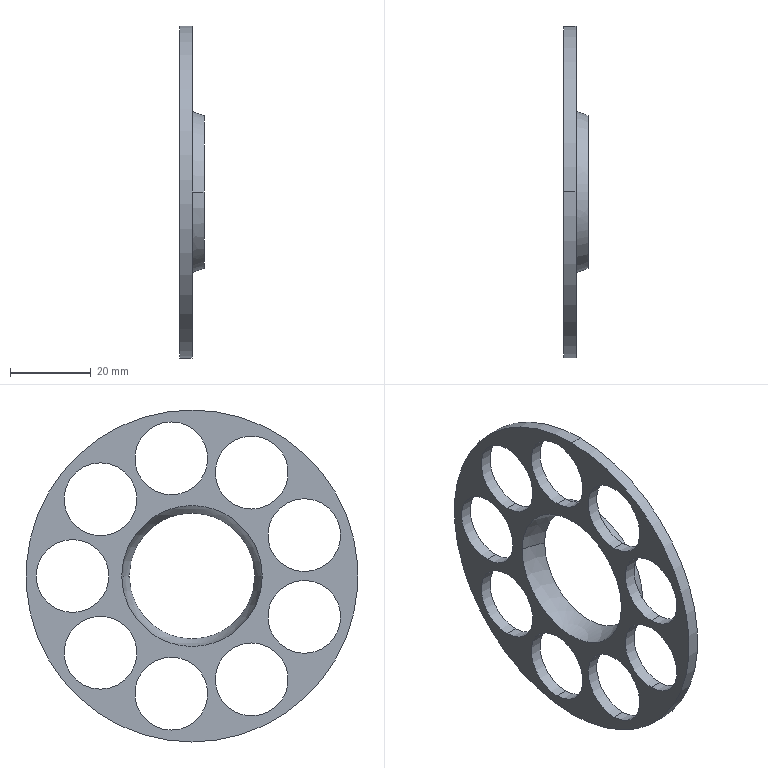Part | SolidWorks | features ICE 1, RevCut 1, Revolution 1 | 1 solid | 27 faces | box 6 x 82 x 82 mm | volume 7292 mm3 | cylinder 20 | sphere 4 | plane 3 | commonest cylinder face diameters 18 x18 82 x2
STEP:
#1=CARTESIAN_POINT('',(0.,5.123,38.052));
#2=VERTEX_POINT('',#1);
#3=CARTESIAN_POINT('',(0.,5.123,20.052));
#4=VERTEX_POINT('',#3);
#5=CARTESIAN_POINT('',(0.,5.123,29.052));
#6=DIRECTION('',(1.,0.,0.));
#7=DIRECTION('',(0.,0.,-1.));
#8=AXIS2_PLACEMENT_3D('',#5,#6,#7);
#9=CIRCLE('',#8,9.);
#10=EDGE_CURVE('',#2,#4,#9,.T.);
#11=ORIENTED_EDGE('',*,*,#10,.F.);
#12=CARTESIAN_POINT('',(3.,5.123,38.052));
#13=VERTEX_POINT('',#12);
#14=CARTESIAN_POINT('',(-7.,5.123,38.052));
#15=DIRECTION('',(1.,0.,0.));
#16=VECTOR('',#15,1000.);
#17=LINE('',#14,#16);
#18=EDGE_CURVE('',#2,#13,#17,.T.);
#19=ORIENTED_EDGE('',*,*,#18,.T.);
#20=CARTESIAN_POINT('',(3.,5.123,20.052));
#21=VERTEX_POINT('',#20);
#22=CARTESIAN_POINT('',(3.,5.123,29.052));
#23=DIRECTION('',(1.,0.,0.));
#24=DIRECTION('',(0.,0.,-1.));
#25=AXIS2_PLACEMENT_3D('',#22,#23,#24);
#26=CIRCLE('',#25,9.);
#27=EDGE_CURVE('',#13,#21,#26,.T.);
#28=ORIENTED_EDGE('',*,*,#27,.T.);
#29=CARTESIAN_POINT('',(-7.,5.123,20.052));
#30=DIRECTION('',(1.,0.,0.));
#31=VECTOR('',#30,1000.);
#32=LINE('',#29,#31);
#33=EDGE_CURVE('',#4,#21,#32,.T.);
#34=ORIENTED_EDGE('',*,*,#33,.F.);
#35=EDGE_LOOP('',(#11,#19,#28,#34));
#36=FACE_OUTER_BOUND('',#35,.T.);
#37=CARTESIAN_POINT('',(-7.,5.123,29.052));
#38=DIRECTION('',(1.,0.,0.));
#39=DIRECTION('',(0.,0.,-1.));
#40=AXIS2_PLACEMENT_3D('',#37,#38,#39);
#41=CYLINDRICAL_SURFACE('',#40,9.);
#42=ADVANCED_FACE('',(#36),#41,.F.);
#43=CARTESIAN_POINT('',(0.,22.598,27.962));
#44=VERTEX_POINT('',#43);
#45=CARTESIAN_POINT('',(0.,22.598,9.962));
#46=VERTEX_POINT('',#45);
#47=CARTESIAN_POINT('',(0.,22.598,18.962));
#48=DIRECTION('',(1.,0.,0.));
#49=DIRECTION('',(0.,0.,-1.));
#50=AXIS2_PLACEMENT_3D('',#47,#48,#49);
#51=CIRCLE('',#50,9.);
#52=EDGE_CURVE('',#44,#46,#51,.T.);
#53=ORIENTED_EDGE('',*,*,#52,.F.);
#54=CARTESIAN_POINT('',(3.,22.598,27.962));
#55=VERTEX_POINT('',#54);
#56=CARTESIAN_POINT('',(-7.,22.598,27.962));
#57=DIRECTION('',(1.,0.,0.));
#58=VECTOR('',#57,1000.);
#59=LINE('',#56,#58);
#60=EDGE_CURVE('',#44,#55,#59,.T.);
#61=ORIENTED_EDGE('',*,*,#60,.T.);
#62=CARTESIAN_POINT('',(3.,22.598,9.962));
#63=VERTEX_POINT('',#62);
#64=CARTESIAN_POINT('',(3.,22.598,18.962));
#65=DIRECTION('',(1.,0.,0.));
#66=DIRECTION('',(0.,0.,-1.));
#67=AXIS2_PLACEMENT_3D('',#64,#65,#66);
#68=CIRCLE('',#67,9.);
#69=EDGE_CURVE('',#55,#63,#68,.T.);
#70=ORIENTED_EDGE('',*,*,#69,.T.);
#71=CARTESIAN_POINT('',(-7.,22.598,9.962));
#72=DIRECTION('',(1.,0.,0.));
#73=VECTOR('',#72,1000.);
#74=LINE('',#71,#73);
#75=EDGE_CURVE('',#46,#63,#74,.T.);
#76=ORIENTED_EDGE('',*,*,#75,.F.);
#77=EDGE_LOOP('',(#53,#61,#70,#76));
#78=FACE_OUTER_BOUND('',#77,.T.);
#79=CARTESIAN_POINT('',(-7.,22.598,18.962));
#80=DIRECTION('',(1.,0.,0.));
#81=DIRECTION('',(0.,0.,-1.));
#82=AXIS2_PLACEMENT_3D('',#79,#80,#81);
#83=CYLINDRICAL_SURFACE('',#82,9.);
#84=ADVANCED_FACE('',(#78),#83,.F.);
#85=CARTESIAN_POINT('',(0.,-27.721,19.09));
#86=VERTEX_POINT('',#85);
#87=CARTESIAN_POINT('',(0.,-27.721,1.09));
#88=VERTEX_POINT('',#87);
#89=CARTESIAN_POINT('',(0.,-27.721,10.09));
#90=DIRECTION('',(1.,0.,0.));
#91=DIRECTION('',(0.,0.,-1.));
#92=AXIS2_PLACEMENT_3D('',#89,#90,#91);
#93=CIRCLE('',#92,9.);
#94=EDGE_CURVE('',#86,#88,#93,.T.);
#95=ORIENTED_EDGE('',*,*,#94,.F.);
#96=CARTESIAN_POINT('',(3.,-27.721,19.09));
#97=VERTEX_POINT('',#96);
#98=CARTESIAN_POINT('',(-7.,-27.721,19.09));
#99=DIRECTION('',(1.,0.,0.));
#100=VECTOR('',#99,1000.);
#101=LINE('',#98,#100);
#102=EDGE_CURVE('',#86,#97,#101,.T.);
#103=ORIENTED_EDGE('',*,*,#102,.T.);
#104=CARTESIAN_POINT('',(3.,-27.721,1.09));
#105=VERTEX_POINT('',#104);
#106=CARTESIAN_POINT('',(3.,-27.721,10.09));
#107=DIRECTION('',(1.,0.,0.));
#108=DIRECTION('',(0.,0.,-1.));
#109=AXIS2_PLACEMENT_3D('',#106,#107,#108);
#110=CIRCLE('',#109,9.);
#111=EDGE_CURVE('',#97,#105,#110,.T.);
#112=ORIENTED_EDGE('',*,*,#111,.T.);
#113=CARTESIAN_POINT('',(-7.,-27.721,1.09));
#114=DIRECTION('',(1.,0.,0.));
#115=VECTOR('',#114,1000.);
#116=LINE('',#113,#115);
#117=EDGE_CURVE('',#88,#105,#116,.T.);
#118=ORIENTED_EDGE('',*,*,#117,.F.);
#119=EDGE_LOOP('',(#95,#103,#112,#118));
#120=FACE_OUTER_BOUND('',#119,.T.);
#121=CARTESIAN_POINT('',(-7.,-27.721,10.09));
#122=DIRECTION('',(1.,0.,0.));
#123=DIRECTION('',(0.,0.,-1.));
#124=AXIS2_PLACEMENT_3D('',#121,#122,#123);
#125=CYLINDRICAL_SURFACE('',#124,9.);
#126=ADVANCED_FACE('',(#120),#125,.F.);
#127=CARTESIAN_POINT('',(0.,-14.75,34.548));
#128=VERTEX_POINT('',#127);
#129=CARTESIAN_POINT('',(0.,-14.75,16.548));
#130=VERTEX_POINT('',#129);
#131=CARTESIAN_POINT('',(0.,-14.75,25.548));
#132=DIRECTION('',(1.,0.,0.));
#133=DIRECTION('',(0.,0.,-1.));
#134=AXIS2_PLACEMENT_3D('',#131,#132,#133);
#135=CIRCLE('',#134,9.);
#136=EDGE_CURVE('',#128,#130,#135,.T.);
#137=ORIENTED_EDGE('',*,*,#136,.F.);
#138=CARTESIAN_POINT('',(3.,-14.75,34.548));
#139=VERTEX_POINT('',#138);
#140=CARTESIAN_POINT('',(-7.,-14.75,34.548));
#141=DIRECTION('',(1.,0.,0.));
#142=VECTOR('',#141,1000.);
#143=LINE('',#140,#142);
#144=EDGE_CURVE('',#128,#139,#143,.T.);
#145=ORIENTED_EDGE('',*,*,#144,.T.);
#146=CARTESIAN_POINT('',(3.,-14.75,16.548));
#147=VERTEX_POINT('',#146);
#148=CARTESIAN_POINT('',(3.,-14.75,25.548));
#149=DIRECTION('',(1.,0.,0.));
#150=DIRECTION('',(0.,0.,-1.));
#151=AXIS2_PLACEMENT_3D('',#148,#149,#150);
#152=CIRCLE('',#151,9.);
#153=EDGE_CURVE('',#139,#147,#152,.T.);
#154=ORIENTED_EDGE('',*,*,#153,.T.);
#155=CARTESIAN_POINT('',(-7.,-14.75,16.548));
#156=DIRECTION('',(1.,0.,0.));
#157=VECTOR('',#156,1000.);
#158=LINE('',#155,#157);
#159=EDGE_CURVE('',#130,#147,#158,.T.);
#160=ORIENTED_EDGE('',*,*,#159,.F.);
#161=EDGE_LOOP('',(#137,#145,#154,#160));
#162=FACE_OUTER_BOUND('',#161,.T.);
#163=CARTESIAN_POINT('',(-7.,-14.75,25.548));
#164=DIRECTION('',(1.,0.,0.));
#165=DIRECTION('',(0.,0.,-1.));
#166=AXIS2_PLACEMENT_3D('',#163,#164,#165);
#167=CYLINDRICAL_SURFACE('',#166,9.);
#168=ADVANCED_FACE('',(#162),#167,.F.);
#169=CARTESIAN_POINT('',(0.,-14.75,-16.548));
#170=VERTEX_POINT('',#169);
#171=CARTESIAN_POINT('',(0.,-14.75,-34.548));
#172=VERTEX_POINT('',#171);
#173=CARTESIAN_POINT('',(0.,-14.75,-25.548));
#174=DIRECTION('',(1.,0.,0.));
#175=DIRECTION('',(0.,0.,-1.));
#176=AXIS2_PLACEMENT_3D('',#173,#174,#175);
#177=CIRCLE('',#176,9.);
#178=EDGE_CURVE('',#170,#172,#177,.T.);
#179=ORIENTED_EDGE('',*,*,#178,.F.);
#180=CARTESIAN_POINT('',(3.,-14.75,-16.548));
#181=VERTEX_POINT('',#180);
#182=CARTESIAN_POINT('',(-7.,-14.75,-16.548));
#183=DIRECTION('',(1.,0.,0.));
#184=VECTOR('',#183,1000.);
#185=LINE('',#182,#184);
#186=EDGE_CURVE('',#170,#181,#185,.T.);
#187=ORIENTED_EDGE('',*,*,#186,.T.);
#188=CARTESIAN_POINT('',(3.,-14.75,-34.548));
#189=VERTEX_POINT('',#188);
#190=CARTESIAN_POINT('',(3.,-14.75,-25.548));
#191=DIRECTION('',(1.,0.,0.));
#192=DIRECTION('',(0.,0.,-1.));
#193=AXIS2_PLACEMENT_3D('',#190,#191,#192);
#194=CIRCLE('',#193,9.);
#195=EDGE_CURVE('',#181,#189,#194,.T.);
#196=ORIENTED_EDGE('',*,*,#195,.T.);
#197=CARTESIAN_POINT('',(-7.,-14.75,-34.548));
#198=DIRECTION('',(1.,0.,0.));
#199=VECTOR('',#198,1000.);
#200=LINE('',#197,#199);
#201=EDGE_CURVE('',#172,#189,#200,.T.);
#202=ORIENTED_EDGE('',*,*,#201,.F.);
#203=EDGE_LOOP('',(#179,#187,#196,#202));
#204=FACE_OUTER_BOUND('',#203,.T.);
#205=CARTESIAN_POINT('',(-7.,-14.75,-25.548));
#206=DIRECTION('',(1.,0.,0.));
#207=DIRECTION('',(0.,0.,-1.));
#208=AXIS2_PLACEMENT_3D('',#205,#206,#207);
#209=CYLINDRICAL_SURFACE('',#208,9.);
#210=ADVANCED_FACE('',(#204),#209,.F.);
#211=CARTESIAN_POINT('',(0.,-27.721,-1.09));
#212=VERTEX_POINT('',#211);
#213=CARTESIAN_POINT('',(0.,-27.721,-19.09));
#214=VERTEX_POINT('',#213);
#215=CARTESIAN_POINT('',(0.,-27.721,-10.09));
#216=DIRECTION('',(1.,0.,0.));
#217=DIRECTION('',(0.,0.,-1.));
#218=AXIS2_PLACEMENT_3D('',#215,#216,#217);
#219=CIRCLE('',#218,9.);
#220=EDGE_CURVE('',#212,#214,#219,.T.);
#221=ORIENTED_EDGE('',*,*,#220,.F.);
#222=CARTESIAN_POINT('',(3.,-27.721,-1.09));
#223=VERTEX_POINT('',#222);
#224=CARTESIAN_POINT('',(-7.,-27.721,-1.09));
#225=DIRECTION('',(1.,0.,0.));
#226=VECTOR('',#225,1000.);
#227=LINE('',#224,#226);
#228=EDGE_CURVE('',#212,#223,#227,.T.);
#229=ORIENTED_EDGE('',*,*,#228,.T.);
#230=CARTESIAN_POINT('',(3.,-27.721,-19.09));
#231=VERTEX_POINT('',#230);
#232=CARTESIAN_POINT('',(3.,-27.721,-10.09));
#233=DIRECTION('',(1.,0.,0.));
#234=DIRECTION('',(0.,0.,-1.));
#235=AXIS2_PLACEMENT_3D('',#232,#233,#234);
#236=CIRCLE('',#235,9.);
#237=EDGE_CURVE('',#223,#231,#236,.T.);
#238=ORIENTED_EDGE('',*,*,#237,.T.);
#239=CARTESIAN_POINT('',(-7.,-27.721,-19.09));
#240=DIRECTION('',(1.,0.,0.));
#241=VECTOR('',#240,1000.);
#242=LINE('',#239,#241);
#243=EDGE_CURVE('',#214,#231,#242,.T.);
#244=ORIENTED_EDGE('',*,*,#243,.F.);
#245=EDGE_LOOP('',(#221,#229,#238,#244));
#246=FACE_OUTER_BOUND('',#245,.T.);
#247=CARTESIAN_POINT('',(-7.,-27.721,-10.09));
#248=DIRECTION('',(1.,0.,0.));
#249=DIRECTION('',(0.,0.,-1.));
#250=AXIS2_PLACEMENT_3D('',#247,#248,#249);
#251=CYLINDRICAL_SURFACE('',#250,9.);
#252=ADVANCED_FACE('',(#246),#251,.F.);
#253=CARTESIAN_POINT('',(0.,22.598,-9.962));
#254=VERTEX_POINT('',#253);
#255=CARTESIAN_POINT('',(0.,22.598,-27.962));
#256=VERTEX_POINT('',#255);
#257=CARTESIAN_POINT('',(0.,22.598,-18.962));
#258=DIRECTION('',(1.,0.,0.));
#259=DIRECTION('',(0.,0.,-1.));
#260=AXIS2_PLACEMENT_3D('',#257,#258,#259);
#261=CIRCLE('',#260,9.);
#262=EDGE_CURVE('',#254,#256,#261,.T.);
#263=ORIENTED_EDGE('',*,*,#262,.F.);
#264=CARTESIAN_POINT('',(3.,22.598,-9.962));
#265=VERTEX_POINT('',#264);
#266=CARTESIAN_POINT('',(-7.,22.598,-9.962));
#267=DIRECTION('',(1.,0.,0.));
#268=VECTOR('',#267,1000.);
#269=LINE('',#266,#268);
#270=EDGE_CURVE('',#254,#265,#269,.T.);
#271=ORIENTED_EDGE('',*,*,#270,.T.);
#272=CARTESIAN_POINT('',(3.,22.598,-27.962));
#273=VERTEX_POINT('',#272);
#274=CARTESIAN_POINT('',(3.,22.598,-18.962));
#275=DIRECTION('',(1.,0.,0.));
#276=DIRECTION('',(0.,0.,-1.));
#277=AXIS2_PLACEMENT_3D('',#274,#275,#276);
#278=CIRCLE('',#277,9.);
#279=EDGE_CURVE('',#265,#273,#278,.T.);
#280=ORIENTED_EDGE('',*,*,#279,.T.);
#281=CARTESIAN_POINT('',(-7.,22.598,-27.962));
#282=DIRECTION('',(1.,0.,0.));
#283=VECTOR('',#282,1000.);
#284=LINE('',#281,#283);
#285=EDGE_CURVE('',#256,#273,#284,.T.);
#286=ORIENTED_EDGE('',*,*,#285,.F.);
#287=EDGE_LOOP('',(#263,#271,#280,#286));
#288=FACE_OUTER_BOUND('',#287,.T.);
#289=CARTESIAN_POINT('',(-7.,22.598,-18.962));
#290=DIRECTION('',(1.,0.,0.));
#291=DIRECTION('',(0.,0.,-1.));
#292=AXIS2_PLACEMENT_3D('',#289,#290,#291);
#293=CYLINDRICAL_SURFACE('',#292,9.);
#294=ADVANCED_FACE('',(#288),#293,.F.);
#295=CARTESIAN_POINT('',(0.,5.123,-20.052));
#296=VERTEX_POINT('',#295);
#297=CARTESIAN_POINT('',(0.,5.123,-38.052));
#298=VERTEX_POINT('',#297);
#299=CARTESIAN_POINT('',(0.,5.123,-29.052));
#300=DIRECTION('',(1.,0.,0.));
#301=DIRECTION('',(0.,0.,-1.));
#302=AXIS2_PLACEMENT_3D('',#299,#300,#301);
#303=CIRCLE('',#302,9.);
#304=EDGE_CURVE('',#296,#298,#303,.T.);
#305=ORIENTED_EDGE('',*,*,#304,.F.);
#306=CARTESIAN_POINT('',(3.,5.123,-20.052));
#307=VERTEX_POINT('',#306);
#308=CARTESIAN_POINT('',(-7.,5.123,-20.052));
#309=DIRECTION('',(1.,0.,0.));
#310=VECTOR('',#309,1000.);
#311=LINE('',#308,#310);
#312=EDGE_CURVE('',#296,#307,#311,.T.);
#313=ORIENTED_EDGE('',*,*,#312,.T.);
#314=CARTESIAN_POINT('',(3.,5.123,-38.052));
#315=VERTEX_POINT('',#314);
#316=CARTESIAN_POINT('',(3.,5.123,-29.052));
#317=DIRECTION('',(1.,0.,0.));
#318=DIRECTION('',(0.,0.,-1.));
#319=AXIS2_PLACEMENT_3D('',#316,#317,#318);
#320=CIRCLE('',#319,9.);
#321=EDGE_CURVE('',#307,#315,#320,.T.);
#322=ORIENTED_EDGE('',*,*,#321,.T.);
#323=CARTESIAN_POINT('',(-7.,5.123,-38.052));
#324=DIRECTION('',(1.,0.,0.));
#325=VECTOR('',#324,1000.);
#326=LINE('',#323,#325);
#327=EDGE_CURVE('',#298,#315,#326,.T.);
#328=ORIENTED_EDGE('',*,*,#327,.F.);
#329=EDGE_LOOP('',(#305,#313,#322,#328));
#330=FACE_OUTER_BOUND('',#329,.T.);
#331=CARTESIAN_POINT('',(-7.,5.123,-29.052));
#332=DIRECTION('',(1.,0.,0.));
#333=DIRECTION('',(0.,0.,-1.));
#334=AXIS2_PLACEMENT_3D('',#331,#332,#333);
#335=CYLINDRICAL_SURFACE('',#334,9.);
#336=ADVANCED_FACE('',(#330),#335,.F.);
#337=CARTESIAN_POINT('',(0.,29.5,9.));
#338=VERTEX_POINT('',#337);
#339=CARTESIAN_POINT('',(0.,29.5,-9.));
#340=VERTEX_POINT('',#339);
#341=CARTESIAN_POINT('',(0.,29.5,0.));
#342=DIRECTION('',(1.,0.,0.));
#343=DIRECTION('',(0.,0.,-1.));
#344=AXIS2_PLACEMENT_3D('',#341,#342,#343);
#345=CIRCLE('',#344,9.);
#346=EDGE_CURVE('',#338,#340,#345,.T.);
#347=ORIENTED_EDGE('',*,*,#346,.F.);
#348=CARTESIAN_POINT('',(3.,29.5,9.));
#349=VERTEX_POINT('',#348);
#350=CARTESIAN_POINT('',(-7.,29.5,9.));
#351=DIRECTION('',(1.,0.,0.));
#352=VECTOR('',#351,1000.);
#353=LINE('',#350,#352);
#354=EDGE_CURVE('',#338,#349,#353,.T.);
#355=ORIENTED_EDGE('',*,*,#354,.T.);
#356=CARTESIAN_POINT('',(3.,29.5,-9.));
#357=VERTEX_POINT('',#356);
#358=CARTESIAN_POINT('',(3.,29.5,0.));
#359=DIRECTION('',(1.,0.,0.));
#360=DIRECTION('',(0.,0.,-1.));
#361=AXIS2_PLACEMENT_3D('',#358,#359,#360);
#362=CIRCLE('',#361,9.);
#363=EDGE_CURVE('',#349,#357,#362,.T.);
#364=ORIENTED_EDGE('',*,*,#363,.T.);
#365=CARTESIAN_POINT('',(-7.,29.5,-9.));
#366=DIRECTION('',(1.,0.,0.));
#367=VECTOR('',#366,1000.);
#368=LINE('',#365,#367);
#369=EDGE_CURVE('',#340,#357,#368,.T.);
#370=ORIENTED_EDGE('',*,*,#369,.F.);
#371=EDGE_LOOP('',(#347,#355,#364,#370));
#372=FACE_OUTER_BOUND('',#371,.T.);
#373=CARTESIAN_POINT('',(-7.,29.5,0.));
#374=DIRECTION('',(1.,0.,0.));
#375=DIRECTION('',(0.,0.,-1.));
#376=AXIS2_PLACEMENT_3D('',#373,#374,#375);
#377=CYLINDRICAL_SURFACE('',#376,9.);
#378=ADVANCED_FACE('',(#372),#377,.F.);
#379=CARTESIAN_POINT('',(0.,-17.371,0.));
#380=VERTEX_POINT('',#379);
#381=CARTESIAN_POINT('',(0.,17.371,0.));
#382=VERTEX_POINT('',#381);
#383=CARTESIAN_POINT('',(0.,0.,0.));
#384=DIRECTION('',(1.,0.,0.));
#385=DIRECTION('',(0.,0.,-1.));
#386=AXIS2_PLACEMENT_3D('',#383,#384,#385);
#387=CIRCLE('',#386,17.371);
#388=EDGE_CURVE('',#380,#382,#387,.T.);
#389=ORIENTED_EDGE('',*,*,#388,.F.);
#390=CARTESIAN_POINT('',(6.,-15.5,0.));
#391=VERTEX_POINT('',#390);
#392=CARTESIAN_POINT('',(-2.124,0.,0.));
#393=DIRECTION('',(0.,0.,1.));
#394=DIRECTION('',(0.,-1.,0.));
#395=AXIS2_PLACEMENT_3D('',#392,#393,#394);
#396=CIRCLE('',#395,17.5);
#397=EDGE_CURVE('',#380,#391,#396,.T.);
#398=ORIENTED_EDGE('',*,*,#397,.T.);
#399=CARTESIAN_POINT('',(6.,15.5,0.));
#400=VERTEX_POINT('',#399);
#401=CARTESIAN_POINT('',(6.,0.,0.));
#402=DIRECTION('',(1.,0.,0.));
#403=DIRECTION('',(0.,0.,-1.));
#404=AXIS2_PLACEMENT_3D('',#401,#402,#403);
#405=CIRCLE('',#404,15.5);
#406=EDGE_CURVE('',#391,#400,#405,.T.);
#407=ORIENTED_EDGE('',*,*,#406,.T.);
#408=CARTESIAN_POINT('',(-2.124,0.,0.));
#409=DIRECTION('',(0.,0.,-1.));
#410=DIRECTION('',(-1.,0.,0.));
#411=AXIS2_PLACEMENT_3D('',#408,#409,#410);
#412=CIRCLE('',#411,17.5);
#413=EDGE_CURVE('',#382,#400,#412,.T.);
#414=ORIENTED_EDGE('',*,*,#413,.F.);
#415=EDGE_LOOP('',(#389,#398,#407,#414));
#416=FACE_OUTER_BOUND('',#415,.T.);
#417=CARTESIAN_POINT('',(-2.124,0.,0.));
#418=DIRECTION('',(0.,0.,1.));
#419=DIRECTION('',(0.,1.,0.));
#420=AXIS2_PLACEMENT_3D('',#417,#418,#419);
#421=SPHERICAL_SURFACE('',#420,17.5);
#422=ADVANCED_FACE('',(#416),#421,.F.);
#423=CARTESIAN_POINT('',(3.,0.,41.));
#424=VERTEX_POINT('',#423);
#425=CARTESIAN_POINT('',(3.,0.,-41.));
#426=VERTEX_POINT('',#425);
#427=CARTESIAN_POINT('',(3.,0.,0.));
#428=DIRECTION('',(-1.,0.,0.));
#429=DIRECTION('',(0.,0.,1.));
#430=AXIS2_PLACEMENT_3D('',#427,#428,#429);
#431=CIRCLE('',#430,41.);
#432=EDGE_CURVE('',#424,#426,#431,.T.);
#433=ORIENTED_EDGE('',*,*,#432,.T.);
#434=CARTESIAN_POINT('',(0.,0.,-41.));
#435=VERTEX_POINT('',#434);
#436=CARTESIAN_POINT('',(0.,0.,-41.));
#437=DIRECTION('',(-1.,0.,0.));
#438=VECTOR('',#437,1000.);
#439=LINE('',#436,#438);
#440=EDGE_CURVE('',#426,#435,#439,.T.);
#441=ORIENTED_EDGE('',*,*,#440,.T.);
#442=CARTESIAN_POINT('',(0.,0.,41.));
#443=VERTEX_POINT('',#442);
#444=CARTESIAN_POINT('',(0.,0.,0.));
#445=DIRECTION('',(-1.,0.,0.));
#446=DIRECTION('',(0.,0.,1.));
#447=AXIS2_PLACEMENT_3D('',#444,#445,#446);
#448=CIRCLE('',#447,41.);
#449=EDGE_CURVE('',#443,#435,#448,.T.);
#450=ORIENTED_EDGE('',*,*,#449,.F.);
#451=CARTESIAN_POINT('',(0.,0.,41.));
#452=DIRECTION('',(-1.,0.,0.));
#453=VECTOR('',#452,1000.);
#454=LINE('',#451,#453);
#455=EDGE_CURVE('',#424,#443,#454,.T.);
#456=ORIENTED_EDGE('',*,*,#455,.F.);
#457=EDGE_LOOP('',(#433,#441,#450,#456));
#458=FACE_OUTER_BOUND('',#457,.T.);
#459=CARTESIAN_POINT('',(0.,0.,0.));
#460=DIRECTION('',(-1.,0.,0.));
#461=DIRECTION('',(0.,0.,1.));
#462=AXIS2_PLACEMENT_3D('',#459,#460,#461);
#463=CYLINDRICAL_SURFACE('',#462,41.);
#464=ADVANCED_FACE('',(#458),#463,.T.);
#465=CARTESIAN_POINT('',(6.,18.822,0.));
#466=VERTEX_POINT('',#465);
#467=CARTESIAN_POINT('',(6.,-18.822,0.));
#468=VERTEX_POINT('',#467);
#469=CARTESIAN_POINT('',(6.,0.,0.));
#470=DIRECTION('',(-1.,0.,0.));
#471=DIRECTION('',(0.,0.,1.));
#472=AXIS2_PLACEMENT_3D('',#469,#470,#471);
#473=CIRCLE('',#472,18.822);
#474=EDGE_CURVE('',#466,#468,#473,.T.);
#475=ORIENTED_EDGE('',*,*,#474,.T.);
#476=CARTESIAN_POINT('',(3.,-19.849,0.));
#477=VERTEX_POINT('',#476);
#478=CARTESIAN_POINT('',(-2.124,0.,0.));
#479=DIRECTION('',(0.,0.,-1.));
#480=DIRECTION('',(0.,1.,0.));
#481=AXIS2_PLACEMENT_3D('',#478,#479,#480);
#482=CIRCLE('',#481,20.5);
#483=EDGE_CURVE('',#468,#477,#482,.T.);
#484=ORIENTED_EDGE('',*,*,#483,.T.);
#485=CARTESIAN_POINT('',(3.,19.849,0.));
#486=VERTEX_POINT('',#485);
#487=CARTESIAN_POINT('',(3.,0.,0.));
#488=DIRECTION('',(-1.,0.,0.));
#489=DIRECTION('',(0.,0.,1.));
#490=AXIS2_PLACEMENT_3D('',#487,#488,#489);
#491=CIRCLE('',#490,19.849);
#492=EDGE_CURVE('',#486,#477,#491,.T.);
#493=ORIENTED_EDGE('',*,*,#492,.F.);
#494=CARTESIAN_POINT('',(-2.124,0.,0.));
#495=DIRECTION('',(0.,0.,1.));
#496=DIRECTION('',(1.,0.,0.));
#497=AXIS2_PLACEMENT_3D('',#494,#495,#496);
#498=CIRCLE('',#497,20.5);
#499=EDGE_CURVE('',#466,#486,#498,.T.);
#500=ORIENTED_EDGE('',*,*,#499,.F.);
#501=EDGE_LOOP('',(#475,#484,#493,#500));
#502=FACE_OUTER_BOUND('',#501,.T.);
#503=CARTESIAN_POINT('',(-2.124,0.,0.));
#504=DIRECTION('',(0.,0.,-1.));
#505=DIRECTION('',(0.,1.,0.));
#506=AXIS2_PLACEMENT_3D('',#503,#504,#505);
#507=SPHERICAL_SURFACE('',#506,20.5);
#508=ADVANCED_FACE('',(#502),#507,.T.);
#509=CARTESIAN_POINT('',(6.,0.,0.));
#510=DIRECTION('',(1.,0.,0.));
#511=DIRECTION('',(0.,0.,-1.));
#512=AXIS2_PLACEMENT_3D('',#509,#510,#511);
#513=CIRCLE('',#512,15.5);
#514=EDGE_CURVE('',#400,#391,#513,.T.);
#515=ORIENTED_EDGE('',*,*,#514,.F.);
#516=ORIENTED_EDGE('',*,*,#406,.F.);
#517=EDGE_LOOP('',(#515,#516));
#518=FACE_BOUND('',#517,.T.);
#519=ORIENTED_EDGE('',*,*,#474,.F.);
#520=CARTESIAN_POINT('',(6.,0.,0.));
#521=DIRECTION('',(-1.,0.,0.));
#522=DIRECTION('',(0.,0.,1.));
#523=AXIS2_PLACEMENT_3D('',#520,#521,#522);
#524=CIRCLE('',#523,18.822);
#525=EDGE_CURVE('',#468,#466,#524,.T.);
#526=ORIENTED_EDGE('',*,*,#525,.F.);
#527=EDGE_LOOP('',(#519,#526));
#528=FACE_OUTER_BOUND('',#527,.T.);
#529=CARTESIAN_POINT('',(6.,0.,0.));
#530=DIRECTION('',(-1.,0.,0.));
#531=DIRECTION('',(0.,0.,1.));
#532=AXIS2_PLACEMENT_3D('',#529,#530,#531);
#533=PLANE('',#532);
#534=ADVANCED_FACE('',(#518,#528),#533,.F.);
#535=ORIENTED_EDGE('',*,*,#483,.F.);
#536=ORIENTED_EDGE('',*,*,#525,.T.);
#537=ORIENTED_EDGE('',*,*,#499,.T.);
#538=CARTESIAN_POINT('',(3.,0.,0.));
#539=DIRECTION('',(-1.,0.,0.));
#540=DIRECTION('',(0.,0.,1.));
#541=AXIS2_PLACEMENT_3D('',#538,#539,#540);
#542=CIRCLE('',#541,19.849);
#543=EDGE_CURVE('',#477,#486,#542,.T.);
#544=ORIENTED_EDGE('',*,*,#543,.F.);
#545=EDGE_LOOP('',(#535,#536,#537,#544));
#546=FACE_OUTER_BOUND('',#545,.T.);
#547=CARTESIAN_POINT('',(-2.124,0.,0.));
#548=DIRECTION('',(0.,0.,-1.));
#549=DIRECTION('',(0.,1.,0.));
#550=AXIS2_PLACEMENT_3D('',#547,#548,#549);
#551=SPHERICAL_SURFACE('',#550,20.5);
#552=ADVANCED_FACE('',(#546),#551,.T.);
#553=CARTESIAN_POINT('',(3.,5.123,29.052));
#554=DIRECTION('',(1.,0.,0.));
#555=DIRECTION('',(0.,0.,-1.));
#556=AXIS2_PLACEMENT_3D('',#553,#554,#555);
#557=CIRCLE('',#556,9.);
#558=EDGE_CURVE('',#21,#13,#557,.T.);
#559=ORIENTED_EDGE('',*,*,#558,.F.);
#560=ORIENTED_EDGE('',*,*,#27,.F.);
#561=EDGE_LOOP('',(#559,#560));
#562=FACE_BOUND('',#561,.T.);
#563=CARTESIAN_POINT('',(3.,22.598,18.962));
#564=DIRECTION('',(1.,0.,0.));
#565=DIRECTION('',(0.,0.,-1.));
#566=AXIS2_PLACEMENT_3D('',#563,#564,#565);
#567=CIRCLE('',#566,9.);
#568=EDGE_CURVE('',#63,#55,#567,.T.);
#569=ORIENTED_EDGE('',*,*,#568,.F.);
#570=ORIENTED_EDGE('',*,*,#69,.F.);
#571=EDGE_LOOP('',(#569,#570));
#572=FACE_BOUND('',#571,.T.);
#573=CARTESIAN_POINT('',(3.,-27.721,10.09));
#574=DIRECTION('',(1.,0.,0.));
#575=DIRECTION('',(0.,0.,-1.));
#576=AXIS2_PLACEMENT_3D('',#573,#574,#575);
#577=CIRCLE('',#576,9.);
#578=EDGE_CURVE('',#105,#97,#577,.T.);
#579=ORIENTED_EDGE('',*,*,#578,.F.);
#580=ORIENTED_EDGE('',*,*,#111,.F.);
#581=EDGE_LOOP('',(#579,#580));
#582=FACE_BOUND('',#581,.T.);
#583=CARTESIAN_POINT('',(3.,-14.75,25.548));
#584=DIRECTION('',(1.,0.,0.));
#585=DIRECTION('',(0.,0.,-1.));
#586=AXIS2_PLACEMENT_3D('',#583,#584,#585);
#587=CIRCLE('',#586,9.);
#588=EDGE_CURVE('',#147,#139,#587,.T.);
#589=ORIENTED_EDGE('',*,*,#588,.F.);
#590=ORIENTED_EDGE('',*,*,#153,.F.);
#591=EDGE_LOOP('',(#589,#590));
#592=FACE_BOUND('',#591,.T.);
#593=CARTESIAN_POINT('',(3.,-14.75,-25.548));
#594=DIRECTION('',(1.,0.,0.));
#595=DIRECTION('',(0.,0.,-1.));
#596=AXIS2_PLACEMENT_3D('',#593,#594,#595);
#597=CIRCLE('',#596,9.);
#598=EDGE_CURVE('',#189,#181,#597,.T.);
#599=ORIENTED_EDGE('',*,*,#598,.F.);
#600=ORIENTED_EDGE('',*,*,#195,.F.);
#601=EDGE_LOOP('',(#599,#600));
#602=FACE_BOUND('',#601,.T.);
#603=CARTESIAN_POINT('',(3.,-27.721,-10.09));
#604=DIRECTION('',(1.,0.,0.));
#605=DIRECTION('',(0.,0.,-1.));
#606=AXIS2_PLACEMENT_3D('',#603,#604,#605);
#607=CIRCLE('',#606,9.);
#608=EDGE_CURVE('',#231,#223,#607,.T.);
#609=ORIENTED_EDGE('',*,*,#608,.F.);
#610=ORIENTED_EDGE('',*,*,#237,.F.);
#611=EDGE_LOOP('',(#609,#610));
#612=FACE_BOUND('',#611,.T.);
#613=CARTESIAN_POINT('',(3.,22.598,-18.962));
#614=DIRECTION('',(1.,0.,0.));
#615=DIRECTION('',(0.,0.,-1.));
#616=AXIS2_PLACEMENT_3D('',#613,#614,#615);
#617=CIRCLE('',#616,9.);
#618=EDGE_CURVE('',#273,#265,#617,.T.);
#619=ORIENTED_EDGE('',*,*,#618,.F.);
#620=ORIENTED_EDGE('',*,*,#279,.F.);
#621=EDGE_LOOP('',(#619,#620));
#622=FACE_BOUND('',#621,.T.);
#623=CARTESIAN_POINT('',(3.,5.123,-29.052));
#624=DIRECTION('',(1.,0.,0.));
#625=DIRECTION('',(0.,0.,-1.));
#626=AXIS2_PLACEMENT_3D('',#623,#624,#625);
#627=CIRCLE('',#626,9.);
#628=EDGE_CURVE('',#315,#307,#627,.T.);
#629=ORIENTED_EDGE('',*,*,#628,.F.);
#630=ORIENTED_EDGE('',*,*,#321,.F.);
#631=EDGE_LOOP('',(#629,#630));
#632=FACE_BOUND('',#631,.T.);
#633=CARTESIAN_POINT('',(3.,29.5,0.));
#634=DIRECTION('',(1.,0.,0.));
#635=DIRECTION('',(0.,0.,-1.));
#636=AXIS2_PLACEMENT_3D('',#633,#634,#635);
#637=CIRCLE('',#636,9.);
#638=EDGE_CURVE('',#357,#349,#637,.T.);
#639=ORIENTED_EDGE('',*,*,#638,.F.);
#640=ORIENTED_EDGE('',*,*,#363,.F.);
#641=EDGE_LOOP('',(#639,#640));
#642=FACE_BOUND('',#641,.T.);
#643=ORIENTED_EDGE('',*,*,#432,.F.);
#644=CARTESIAN_POINT('',(3.,0.,0.));
#645=DIRECTION('',(-1.,0.,0.));
#646=DIRECTION('',(0.,0.,1.));
#647=AXIS2_PLACEMENT_3D('',#644,#645,#646);
#648=CIRCLE('',#647,41.);
#649=EDGE_CURVE('',#426,#424,#648,.T.);
#650=ORIENTED_EDGE('',*,*,#649,.F.);
#651=EDGE_LOOP('',(#643,#650));
#652=FACE_OUTER_BOUND('',#651,.T.);
#653=ORIENTED_EDGE('',*,*,#492,.T.);
#654=ORIENTED_EDGE('',*,*,#543,.T.);
#655=EDGE_LOOP('',(#653,#654));
#656=FACE_BOUND('',#655,.T.);
#657=CARTESIAN_POINT('',(3.,19.849,0.));
#658=DIRECTION('',(-1.,0.,0.));
#659=DIRECTION('',(0.,0.,1.));
#660=AXIS2_PLACEMENT_3D('',#657,#658,#659);
#661=PLANE('',#660);
#662=ADVANCED_FACE('',(#562,#572,#582,#592,#602,#612,#622,#632,#642,#652,#656),#661,.F.);
#663=ORIENTED_EDGE('',*,*,#440,.F.);
#664=ORIENTED_EDGE('',*,*,#649,.T.);
#665=ORIENTED_EDGE('',*,*,#455,.T.);
#666=CARTESIAN_POINT('',(0.,0.,0.));
#667=DIRECTION('',(-1.,0.,0.));
#668=DIRECTION('',(0.,0.,1.));
#669=AXIS2_PLACEMENT_3D('',#666,#667,#668);
#670=CIRCLE('',#669,41.);
#671=EDGE_CURVE('',#435,#443,#670,.T.);
#672=ORIENTED_EDGE('',*,*,#671,.F.);
#673=EDGE_LOOP('',(#663,#664,#665,#672));
#674=FACE_OUTER_BOUND('',#673,.T.);
#675=CARTESIAN_POINT('',(0.,0.,0.));
#676=DIRECTION('',(-1.,0.,0.));
#677=DIRECTION('',(0.,0.,1.));
#678=AXIS2_PLACEMENT_3D('',#675,#676,#677);
#679=CYLINDRICAL_SURFACE('',#678,41.);
#680=ADVANCED_FACE('',(#674),#679,.T.);
#681=CARTESIAN_POINT('',(0.,5.123,29.052));
#682=DIRECTION('',(1.,0.,0.));
#683=DIRECTION('',(0.,0.,-1.));
#684=AXIS2_PLACEMENT_3D('',#681,#682,#683);
#685=CIRCLE('',#684,9.);
#686=EDGE_CURVE('',#4,#2,#685,.T.);
#687=ORIENTED_EDGE('',*,*,#686,.T.);
#688=ORIENTED_EDGE('',*,*,#10,.T.);
#689=EDGE_LOOP('',(#687,#688));
#690=FACE_BOUND('',#689,.T.);
#691=CARTESIAN_POINT('',(0.,22.598,18.962));
#692=DIRECTION('',(1.,0.,0.));
#693=DIRECTION('',(0.,0.,-1.));
#694=AXIS2_PLACEMENT_3D('',#691,#692,#693);
#695=CIRCLE('',#694,9.);
#696=EDGE_CURVE('',#46,#44,#695,.T.);
#697=ORIENTED_EDGE('',*,*,#696,.T.);
#698=ORIENTED_EDGE('',*,*,#52,.T.);
#699=EDGE_LOOP('',(#697,#698));
#700=FACE_BOUND('',#699,.T.);
#701=CARTESIAN_POINT('',(0.,-27.721,10.09));
#702=DIRECTION('',(1.,0.,0.));
#703=DIRECTION('',(0.,0.,-1.));
#704=AXIS2_PLACEMENT_3D('',#701,#702,#703);
#705=CIRCLE('',#704,9.);
#706=EDGE_CURVE('',#88,#86,#705,.T.);
#707=ORIENTED_EDGE('',*,*,#706,.T.);
#708=ORIENTED_EDGE('',*,*,#94,.T.);
#709=EDGE_LOOP('',(#707,#708));
#710=FACE_BOUND('',#709,.T.);
#711=CARTESIAN_POINT('',(0.,-14.75,25.548));
#712=DIRECTION('',(1.,0.,0.));
#713=DIRECTION('',(0.,0.,-1.));
#714=AXIS2_PLACEMENT_3D('',#711,#712,#713);
#715=CIRCLE('',#714,9.);
#716=EDGE_CURVE('',#130,#128,#715,.T.);
#717=ORIENTED_EDGE('',*,*,#716,.T.);
#718=ORIENTED_EDGE('',*,*,#136,.T.);
#719=EDGE_LOOP('',(#717,#718));
#720=FACE_BOUND('',#719,.T.);
#721=CARTESIAN_POINT('',(0.,-14.75,-25.548));
#722=DIRECTION('',(1.,0.,0.));
#723=DIRECTION('',(0.,0.,-1.));
#724=AXIS2_PLACEMENT_3D('',#721,#722,#723);
#725=CIRCLE('',#724,9.);
#726=EDGE_CURVE('',#172,#170,#725,.T.);
#727=ORIENTED_EDGE('',*,*,#726,.T.);
#728=ORIENTED_EDGE('',*,*,#178,.T.);
#729=EDGE_LOOP('',(#727,#728));
#730=FACE_BOUND('',#729,.T.);
#731=CARTESIAN_POINT('',(0.,-27.721,-10.09));
#732=DIRECTION('',(1.,0.,0.));
#733=DIRECTION('',(0.,0.,-1.));
#734=AXIS2_PLACEMENT_3D('',#731,#732,#733);
#735=CIRCLE('',#734,9.);
#736=EDGE_CURVE('',#214,#212,#735,.T.);
#737=ORIENTED_EDGE('',*,*,#736,.T.);
#738=ORIENTED_EDGE('',*,*,#220,.T.);
#739=EDGE_LOOP('',(#737,#738));
#740=FACE_BOUND('',#739,.T.);
#741=CARTESIAN_POINT('',(0.,22.598,-18.962));
#742=DIRECTION('',(1.,0.,0.));
#743=DIRECTION('',(0.,0.,-1.));
#744=AXIS2_PLACEMENT_3D('',#741,#742,#743);
#745=CIRCLE('',#744,9.);
#746=EDGE_CURVE('',#256,#254,#745,.T.);
#747=ORIENTED_EDGE('',*,*,#746,.T.);
#748=ORIENTED_EDGE('',*,*,#262,.T.);
#749=EDGE_LOOP('',(#747,#748));
#750=FACE_BOUND('',#749,.T.);
#751=CARTESIAN_POINT('',(0.,5.123,-29.052));
#752=DIRECTION('',(1.,0.,0.));
#753=DIRECTION('',(0.,0.,-1.));
#754=AXIS2_PLACEMENT_3D('',#751,#752,#753);
#755=CIRCLE('',#754,9.);
#756=EDGE_CURVE('',#298,#296,#755,.T.);
#757=ORIENTED_EDGE('',*,*,#756,.T.);
#758=ORIENTED_EDGE('',*,*,#304,.T.);
#759=EDGE_LOOP('',(#757,#758));
#760=FACE_BOUND('',#759,.T.);
#761=CARTESIAN_POINT('',(0.,29.5,0.));
#762=DIRECTION('',(1.,0.,0.));
#763=DIRECTION('',(0.,0.,-1.));
#764=AXIS2_PLACEMENT_3D('',#761,#762,#763);
#765=CIRCLE('',#764,9.);
#766=EDGE_CURVE('',#340,#338,#765,.T.);
#767=ORIENTED_EDGE('',*,*,#766,.T.);
#768=ORIENTED_EDGE('',*,*,#346,.T.);
#769=EDGE_LOOP('',(#767,#768));
#770=FACE_BOUND('',#769,.T.);
#771=CARTESIAN_POINT('',(0.,0.,0.));
#772=DIRECTION('',(1.,0.,0.));
#773=DIRECTION('',(0.,0.,-1.));
#774=AXIS2_PLACEMENT_3D('',#771,#772,#773);
#775=CIRCLE('',#774,17.371);
#776=EDGE_CURVE('',#382,#380,#775,.T.);
#777=ORIENTED_EDGE('',*,*,#776,.T.);
#778=ORIENTED_EDGE('',*,*,#388,.T.);
#779=EDGE_LOOP('',(#777,#778));
#780=FACE_BOUND('',#779,.T.);
#781=ORIENTED_EDGE('',*,*,#449,.T.);
#782=ORIENTED_EDGE('',*,*,#671,.T.);
#783=EDGE_LOOP('',(#781,#782));
#784=FACE_OUTER_BOUND('',#783,.T.);
#785=CARTESIAN_POINT('',(0.,41.,0.));
#786=DIRECTION('',(1.,0.,0.));
#787=DIRECTION('',(0.,0.,-1.));
#788=AXIS2_PLACEMENT_3D('',#785,#786,#787);
#789=PLANE('',#788);
#790=ADVANCED_FACE('',(#690,#700,#710,#720,#730,#740,#750,#760,#770,#780,#784),#789,.F.);
#791=ORIENTED_EDGE('',*,*,#397,.F.);
#792=ORIENTED_EDGE('',*,*,#776,.F.);
#793=ORIENTED_EDGE('',*,*,#413,.T.);
#794=ORIENTED_EDGE('',*,*,#514,.T.);
#795=EDGE_LOOP('',(#791,#792,#793,#794));
#796=FACE_OUTER_BOUND('',#795,.T.);
#797=CARTESIAN_POINT('',(-2.124,0.,0.));
#798=DIRECTION('',(0.,0.,1.));
#799=DIRECTION('',(0.,1.,0.));
#800=AXIS2_PLACEMENT_3D('',#797,#798,#799);
#801=SPHERICAL_SURFACE('',#800,17.5);
#802=ADVANCED_FACE('',(#796),#801,.F.);
#803=ORIENTED_EDGE('',*,*,#354,.F.);
#804=ORIENTED_EDGE('',*,*,#766,.F.);
#805=ORIENTED_EDGE('',*,*,#369,.T.);
#806=ORIENTED_EDGE('',*,*,#638,.T.);
#807=EDGE_LOOP('',(#803,#804,#805,#806));
#808=FACE_OUTER_BOUND('',#807,.T.);
#809=CARTESIAN_POINT('',(-7.,29.5,0.));
#810=DIRECTION('',(1.,0.,0.));
#811=DIRECTION('',(0.,0.,-1.));
#812=AXIS2_PLACEMENT_3D('',#809,#810,#811);
#813=CYLINDRICAL_SURFACE('',#812,9.);
#814=ADVANCED_FACE('',(#808),#813,.F.);
#815=ORIENTED_EDGE('',*,*,#312,.F.);
#816=ORIENTED_EDGE('',*,*,#756,.F.);
#817=ORIENTED_EDGE('',*,*,#327,.T.);
#818=ORIENTED_EDGE('',*,*,#628,.T.);
#819=EDGE_LOOP('',(#815,#816,#817,#818));
#820=FACE_OUTER_BOUND('',#819,.T.);
#821=CARTESIAN_POINT('',(-7.,5.123,-29.052));
#822=DIRECTION('',(1.,0.,0.));
#823=DIRECTION('',(0.,0.,-1.));
#824=AXIS2_PLACEMENT_3D('',#821,#822,#823);
#825=CYLINDRICAL_SURFACE('',#824,9.);
#826=ADVANCED_FACE('',(#820),#825,.F.);
#827=ORIENTED_EDGE('',*,*,#270,.F.);
#828=ORIENTED_EDGE('',*,*,#746,.F.);
#829=ORIENTED_EDGE('',*,*,#285,.T.);
#830=ORIENTED_EDGE('',*,*,#618,.T.);
#831=EDGE_LOOP('',(#827,#828,#829,#830));
#832=FACE_OUTER_BOUND('',#831,.T.);
#833=CARTESIAN_POINT('',(-7.,22.598,-18.962));
#834=DIRECTION('',(1.,0.,0.));
#835=DIRECTION('',(0.,0.,-1.));
#836=AXIS2_PLACEMENT_3D('',#833,#834,#835);
#837=CYLINDRICAL_SURFACE('',#836,9.);
#838=ADVANCED_FACE('',(#832),#837,.F.);
#839=ORIENTED_EDGE('',*,*,#228,.F.);
#840=ORIENTED_EDGE('',*,*,#736,.F.);
#841=ORIENTED_EDGE('',*,*,#243,.T.);
#842=ORIENTED_EDGE('',*,*,#608,.T.);
#843=EDGE_LOOP('',(#839,#840,#841,#842));
#844=FACE_OUTER_BOUND('',#843,.T.);
#845=CARTESIAN_POINT('',(-7.,-27.721,-10.09));
#846=DIRECTION('',(1.,0.,0.));
#847=DIRECTION('',(0.,0.,-1.));
#848=AXIS2_PLACEMENT_3D('',#845,#846,#847);
#849=CYLINDRICAL_SURFACE('',#848,9.);
#850=ADVANCED_FACE('',(#844),#849,.F.);
#851=ORIENTED_EDGE('',*,*,#186,.F.);
#852=ORIENTED_EDGE('',*,*,#726,.F.);
#853=ORIENTED_EDGE('',*,*,#201,.T.);
#854=ORIENTED_EDGE('',*,*,#598,.T.);
#855=EDGE_LOOP('',(#851,#852,#853,#854));
#856=FACE_OUTER_BOUND('',#855,.T.);
#857=CARTESIAN_POINT('',(-7.,-14.75,-25.548));
#858=DIRECTION('',(1.,0.,0.));
#859=DIRECTION('',(0.,0.,-1.));
#860=AXIS2_PLACEMENT_3D('',#857,#858,#859);
#861=CYLINDRICAL_SURFACE('',#860,9.);
#862=ADVANCED_FACE('',(#856),#861,.F.);
#863=ORIENTED_EDGE('',*,*,#144,.F.);
#864=ORIENTED_EDGE('',*,*,#716,.F.);
#865=ORIENTED_EDGE('',*,*,#159,.T.);
#866=ORIENTED_EDGE('',*,*,#588,.T.);
#867=EDGE_LOOP('',(#863,#864,#865,#866));
#868=FACE_OUTER_BOUND('',#867,.T.);
#869=CARTESIAN_POINT('',(-7.,-14.75,25.548));
#870=DIRECTION('',(1.,0.,0.));
#871=DIRECTION('',(0.,0.,-1.));
#872=AXIS2_PLACEMENT_3D('',#869,#870,#871);
#873=CYLINDRICAL_SURFACE('',#872,9.);
#874=ADVANCED_FACE('',(#868),#873,.F.);
#875=ORIENTED_EDGE('',*,*,#102,.F.);
#876=ORIENTED_EDGE('',*,*,#706,.F.);
#877=ORIENTED_EDGE('',*,*,#117,.T.);
#878=ORIENTED_EDGE('',*,*,#578,.T.);
#879=EDGE_LOOP('',(#875,#876,#877,#878));
#880=FACE_OUTER_BOUND('',#879,.T.);
#881=CARTESIAN_POINT('',(-7.,-27.721,10.09));
#882=DIRECTION('',(1.,0.,0.));
#883=DIRECTION('',(0.,0.,-1.));
#884=AXIS2_PLACEMENT_3D('',#881,#882,#883);
#885=CYLINDRICAL_SURFACE('',#884,9.);
#886=ADVANCED_FACE('',(#880),#885,.F.);
#887=ORIENTED_EDGE('',*,*,#60,.F.);
#888=ORIENTED_EDGE('',*,*,#696,.F.);
#889=ORIENTED_EDGE('',*,*,#75,.T.);
#890=ORIENTED_EDGE('',*,*,#568,.T.);
#891=EDGE_LOOP('',(#887,#888,#889,#890));
#892=FACE_OUTER_BOUND('',#891,.T.);
#893=CARTESIAN_POINT('',(-7.,22.598,18.962));
#894=DIRECTION('',(1.,0.,0.));
#895=DIRECTION('',(0.,0.,-1.));
#896=AXIS2_PLACEMENT_3D('',#893,#894,#895);
#897=CYLINDRICAL_SURFACE('',#896,9.);
#898=ADVANCED_FACE('',(#892),#897,.F.);
#899=ORIENTED_EDGE('',*,*,#18,.F.);
#900=ORIENTED_EDGE('',*,*,#686,.F.);
#901=ORIENTED_EDGE('',*,*,#33,.T.);
#902=ORIENTED_EDGE('',*,*,#558,.T.);
#903=EDGE_LOOP('',(#899,#900,#901,#902));
#904=FACE_OUTER_BOUND('',#903,.T.);
#905=CARTESIAN_POINT('',(-7.,5.123,29.052));
#906=DIRECTION('',(1.,0.,0.));
#907=DIRECTION('',(0.,0.,-1.));
#908=AXIS2_PLACEMENT_3D('',#905,#906,#907);
#909=CYLINDRICAL_SURFACE('',#908,9.);
#910=ADVANCED_FACE('',(#904),#909,.F.);
#911=CLOSED_SHELL('',(#42,#84,#126,#168,#210,#252,#294,#336,#378,#422,#464,#508,#534,#552,#662,#680,#790,#802,#814,#826,#838,#850,#862,#874,#886,#898,#910));
#912=MANIFOLD_SOLID_BREP('',#911);
#913=CARTESIAN_POINT('',(0.,0.,0.));
#914=DIRECTION('',(0.,0.,1.));
#915=DIRECTION('',(1.,0.,0.));
#916=AXIS2_PLACEMENT_3D('',#913,#914,#915);
#917=(LENGTH_UNIT()NAMED_UNIT(*)SI_UNIT(.MILLI.,.METRE.));
#918=UNCERTAINTY_MEASURE_WITH_UNIT(LENGTH_MEASURE(0.00001),#917,'','');
#919=(NAMED_UNIT(*)PLANE_ANGLE_UNIT()SI_UNIT($,.RADIAN.));
#920=(NAMED_UNIT(*)SI_UNIT($,.STERADIAN.)SOLID_ANGLE_UNIT());
#921=(GEOMETRIC_REPRESENTATION_CONTEXT(3)GLOBAL_UNCERTAINTY_ASSIGNED_CONTEXT((#918))GLOBAL_UNIT_ASSIGNED_CONTEXT((#917,#919,#920))REPRESENTATION_CONTEXT('',''));
#922=ADVANCED_BREP_SHAPE_REPRESENTATION('',(#912,#916),#921);